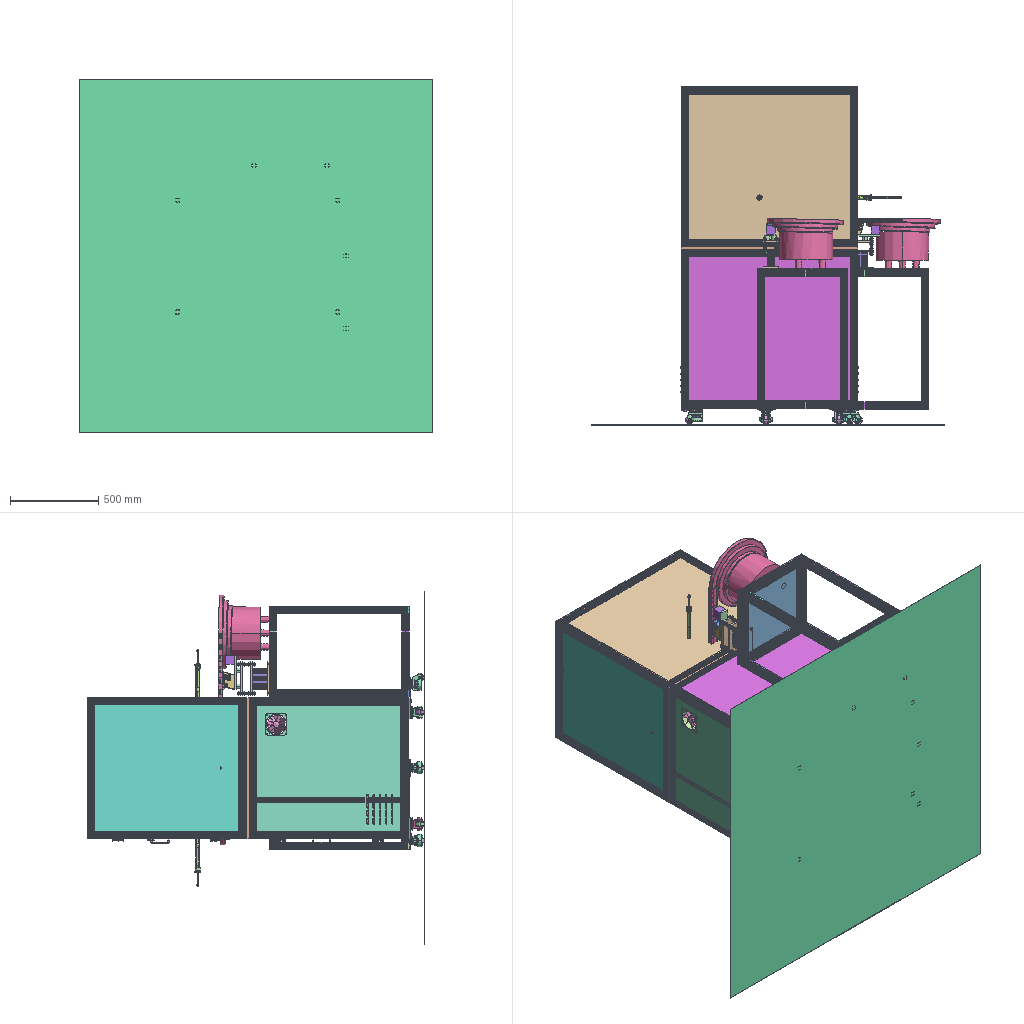Assembly | STEP file | 130 different items | 445 placed | box 2000 x 1911 x 2000 mm
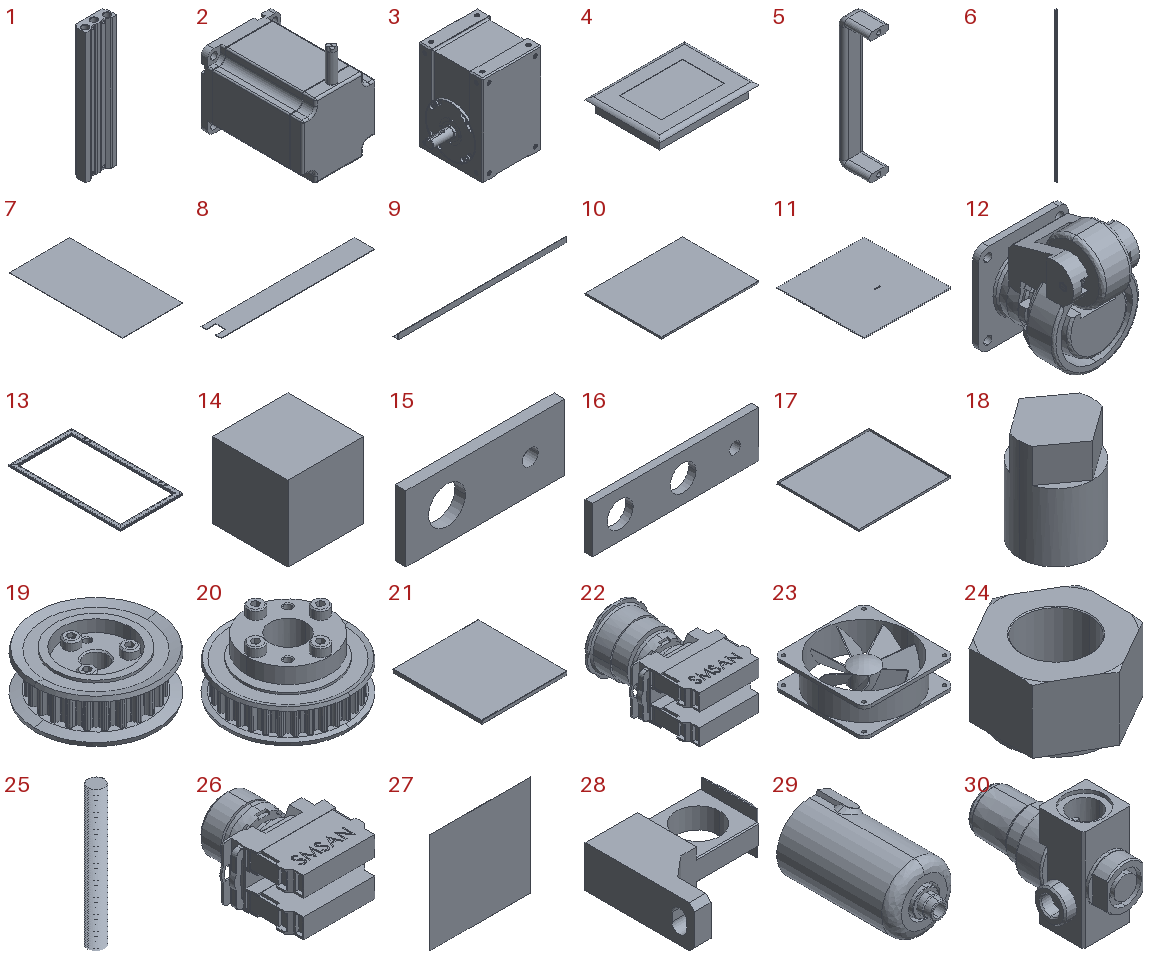Parts list (item | name | quantity | parent item | size | volume):
1 | 200M10F AirTAC base | x1 | in Solenoid valve group | 60 x 24 x 251 mm | 220028 mm3
2 | 57系列三相混合式步进电机[573S15]大国工匠 | x1 | in Material mechanism | 57.15 x 100 x 81.15 mm | 232236 mm3
3 | 60DF cam indexer | x1 | in Material mechanism | 190 x 140 x 170 mm | 2161358 mm3
4 | 7-inch Weintek touch screen TH765-N[7-inch Weintek touch screen TH765-N]_7-inch Weintek touch screen TH765-N | x1 | in Frame assembly | 213 x 159 x 46.5 mm | 1006657 mm3
5 | AKM01-96 handle | x3 | in Frame assembly | 15.6 x 25 x 102 mm | 11694 mm3
6 | AMH71封条-408 | x2 | in Frame assembly | 10.8 x 17.5 x 720 mm | 56736 mm3
7 | Acrylic cabinet door | x3 | in Frame assembly | 418.495 x 778.997 x 2 mm | 652013 mm3
8 | Acrylic cover plate | x2 | in Vibratory feeder mechanism, Vibratory feeder mechanism- | 315 x 41 x 1 mm | 12515 mm3
9 | Angle steel_Default<machined> | x2 | in Frame assembly | 960 x 30 x 30 mm | 210971 mm3
10 | Base plate | x1 | in Frame assembly | 919 x 719 x 16.2 mm | 850250 mm3
11 | Bass plate | x1 | in Material mechanism | 800 x 800 x 8 mm | 5115227 mm3
12 | CGR51-60-U Fuma caster | x2 | in Frame assembly | 73 x 81.5 x 99 mm | 226029 mm3
13 | Cabinet door_Default<machined> | x1 | in Frame assembly | 457.5 x 818 x 15 mm | 630876 mm3
14 | Collection box | x1 | in Hinge assembly equipment | 150 x 150 x 150 mm | 220232 mm3
15 | Connecting plate | x2 | in Handling mechanism | 60 x 4 x 25 mm | 5271 mm3
16 | Connecting plate 2 | x1 | in Station 4 mechanism | 90 x 4 x 25 mm | 7655 mm3
17 | Cover plate | x1 | in Frame assembly | 918 x 818 x 20 mm | 977655 mm3
18 | Diamond pin | x8 | in Material mechanism | 6.5 x 6.5 x 9 mm | 250.881 mm3
19 | ECC05-S5M100-24-F-d8 stepper motor timing pulley | x1 | in Material mechanism | 45 x 45 x 16 mm | 14077 mm3
20 | ECC05-S5M100-32-E-d16 | x1 | in Material mechanism | 55 x 55 x 29 mm | 33207 mm3
21 | Electrical plate | x1 | in Frame assembly | 337.193 x 351.476 x 13.2 mm | 161258 mm3
22 | Emergency stop button[QG115-A1-01ZS╱R] | x1 | in Frame assembly | 48.3 x 74.961 x 39.345 mm | 58947 mm3
23 | Fan[Fan]_Fan | x2 | in Frame assembly | 120 x 120 x 40.344 mm | 86776 mm3
24 | GB/T1229-1991 high-strength heavy hex nut for steel structures M12 | x32 | in Vibratory feeder mechanism, Vibratory feeder mechanism- | 19.773 x 22.78 x 12.3 mm | 2715 mm3
25 | GB/T15389-1994 screw rod M12×100 | x8 | in Vibratory feeder mechanism, Vibratory feeder mechanism- | 12 x 12 x 100 mm | 9042 mm3
26 | Green button[QG115-A2-10TD╱G] | x1 | in Frame assembly | 48.3 x 61.9 x 30.1 mm | 44921 mm3
27 | Ground | x1 | in Hinge assembly equipment | 2000 x 2 x 2000 mm | 8000000 mm3
28 | HI_BC4000 Br | x2 | in BC4000 (FRL unit) | 60 x 52.5 x 20 mm | 24751 mm3
29 | HI_BF4000-A By | x1 | in BC4000 (FRL unit) | 54.5 x 108 x 57.228 mm | 40033 mm3
30 | HI_BR4000 By-BR | x1 | in BC4000 (FRL unit) | 44 x 86.3 x 63 mm | 87528 mm3
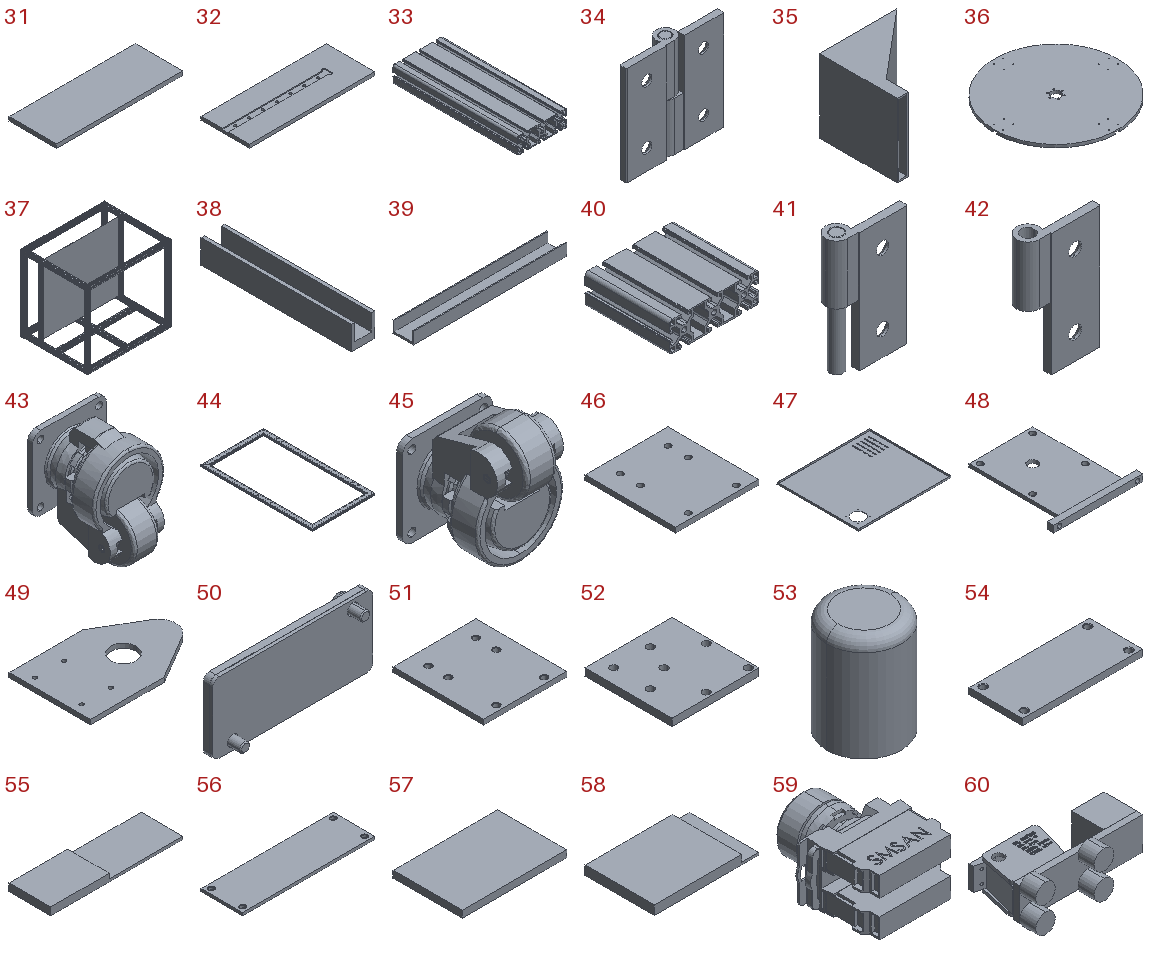31 | Handling mechanism base plate | x3 | in Handling mechanism, Station 4 mechanism | 160 x 60 x 5 mm | 48000 mm3
32 | Handling mechanism support plate | x3 | in Handling mechanism, Station 4 mechanism | 181.74 x 70 x 5 mm | 61345 mm3
33 | Handling mechanism support_Default<machined> | x3 | in Handling mechanism, Station 4 mechanism | 120 x 300 x 40 mm | 478423 mm3
34 | Hinge assembly | x2 | in Hinge assembly equipment, Material mechanism | 62 x 12.05 x 63 mm | 18899 mm3
35 | Hopper | x1 | in Station 3 mechanism | 69.588 x 70 x 66 mm | 22407 mm3
36 | Indexing plate | x1 | in Material mechanism | 450 x 450 x 12 mm | 1702254 mm3
37 | Lower frame_aluminium extrusion<machined> | x1 | in Frame assembly | 1000 x 800 x 900 mm | 9363602 mm3
38 | Magazine box | x1 | in Station 3 mechanism | 10 x 63 x 10 mm | 3213 mm3
39 | Material chute | x2 | in Vibratory feeder mechanism, Vibratory feeder mechanism- | 315 x 41 x 24 mm | 76860 mm3
40 | Material transfer mechanism support_Default<machined> | x2 | in Material transfer mechanism, Material transfer mechanism- | 120 x 112.995 x 40 mm | 180199 mm3
41 | Mirror _AKQ01-B-Z-R-6263-001 | x2 | in Mirrored AKQ01 hinge | 36.75 x 12.05 x 63 mm | 10659 mm3
42 | Mirror _AKQ01-B-Z-R-6263-002 | x2 | in Mirrored AKQ01 hinge | 36.75 x 12.05 x 63 mm | 8240 mm3
43 | Mirrored CGR51-60-U Fuma caster | x1 | in Frame assembly | 73 x 81.5 x 99 mm | 226024 mm3
44 | Mirrored cabinet door_Default<machined> | x2 | in Frame assembly | 457.5 x 818 x 15 mm | 630876 mm3
45 | Mirrored mirrored CGR51-60-U Fuma caster | x1 | in Frame assembly | 73 x 81.5 x 99 mm | 226029 mm3
46 | Mirrored pad plate | x2 | in Vibratory bowl feeder support mechanism | 100.5 x 110 x 6 mm | 64996 mm3
47 | Mirrored side cover plate1_mirror | x1 | in Frame assembly | 818 x 718 x 22.2 mm | 748491 mm3
48 | Motor mounting plate | x1 | in Material mechanism | 80 x 87.326 x 6 mm | 16246 mm3
49 | Mounting plate | x3 | in Handling mechanism, Station 4 mechanism | 108.5 x 70 x 4 mm | 23874 mm3
50 | P-200M-R2 AirTAC base blind plate assembly | x1 | in Solenoid valve group | 50.7 x 9 x 22.4 mm | 3480 mm3
51 | Pad plate | x2 | in Vibratory bowl feeder support mechanism | 100.5 x 110 x 6 mm | 64996 mm3
52 | Pad plate- | x4 | in Frame assembly | 120 x 120 x 10 mm | 138500 mm3
53 | Pin | x8 | in Material mechanism | 6.5 x 6.5 x 9 mm | 259.622 mm3
54 | Plate | x6 | in Vibratory feeder mechanism, Vibratory feeder mechanism- | 190 x 85 x 10 mm | 158173 mm3
55 | Plate 1 | x2 | in Material transfer mechanism, Material transfer mechanism- | 190 x 60 x 11 mm | 80880 mm3
56 | Plate 2 | x2 | in Material transfer mechanism, Material transfer mechanism- | 190 x 60 x 4 mm | 45001 mm3
57 | Plate 3 | x1 | in Station 3 mechanism | 91 x 60 x 6 mm | 32760 mm3
58 | Plate 4 | x1 | in Station 3 mechanism | 91 x 60 x 8 mm | 38280 mm3
59 | Red button[QG115-A2-10TD╱R] | x1 | in Frame assembly | 48.3 x 61.9 x 30.1 mm | 44921 mm3
60 | SKC-PZ-100 counterweight vibratory feeder | x2 | in Vibratory feeder mechanism, Vibratory feeder mechanism- | - | 385547 mm3
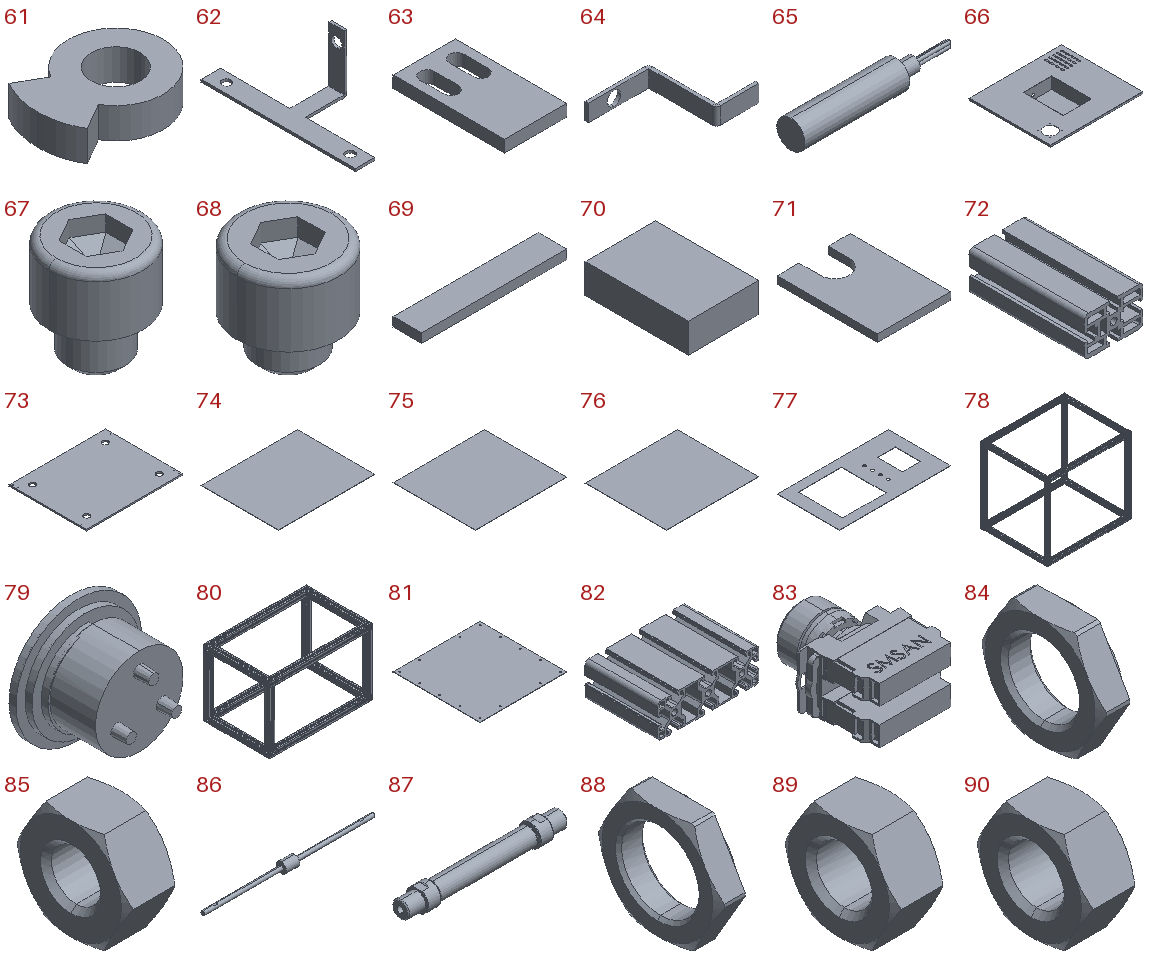61 | Sensing plate | x1 | in Material mechanism | 41 x 31 x 10 mm | 7684 mm3
62 | Sensor bracket | x1 | in Material mechanism | 47.2 x 120 x 45 mm | 5138 mm3
63 | Sensor spacer block | x2 | in Material transfer mechanism, Material transfer mechanism- | 21 x 37.576 x 4 mm | 2679 mm3
64 | Sensor support | x2 | in Material transfer mechanism, Material transfer mechanism- | 60.39 x 42 x 10 mm | 1887 mm3
65 | Sensors | x3 | in Material mechanism, Material transfer mechanism, Material transfer mechanism- | 45 x 8 x 8 mm | 1594 mm3
66 | Side cover plate | x1 | in Frame assembly | 818 x 718 x 108.6 mm | 888983 mm3
67 | Socket head cap screw M10x8 | x12 | in Frame assembly | 16 x 16 x 18 mm | 2409 mm3
68 | Socket head cap screw M8x5 | x16 | in Frame assembly | 13 x 13 x 13 mm | 1204 mm3
69 | Spacer block | x2 | in Station 1 feeding mechanism, Station 2 mechanism | 126 x 24.75 x 7.95 mm | 24792 mm3
70 | Spacer block 4 | x3 | in Handling mechanism, Station 4 mechanism | 48 x 70 x 20 mm | 67200 mm3
71 | Station 3 cylinder connecting plate | x1 | in Station 3 mechanism | 40 x 55 x 4 mm | 7662 mm3
72 | Station 3 support_Default<machined> | x1 | in Station 3 mechanism | 60 x 118.295 x 40 mm | 132045 mm3
73 | Top plate | x1 | in Frame assembly | 1000 x 800 x 14 mm | 11039590 mm3
74 | Upper cover plate | x1 | in Frame assembly | 1000 x 800 x 3 mm | 2399999 mm3
75 | Upper frame acrylic cover plate | x1 | in Frame assembly | 948.003 x 848 x 2 mm | 1607813 mm3
76 | Upper frame acrylic side plate | x2 | in Frame assembly | 848.001 x 747.917 x 2 mm | 1268468 mm3
77 | Upper frame door panel | x1 | in Frame assembly | 848 x 474.5 x 2 mm | 525505 mm3
78 | Upper frame_Default<machined> | x1 | in Frame assembly | 1000 x 800 x 900 mm | 6810900 mm3
79 | Vibratory bowl feeder | x2 | in Station 1 feeding mechanism, Station 2 mechanism | 416.592 x 286.08 x 431.538 mm | 12004626 mm3
80 | Vibratory bowl feeder support frame_Default<machined> | x2 | in Vibratory bowl feeder support mechanism | 790 x 510 x 510 mm | 4425071 mm3
81 | Vibratory bowl feeder support plate | x2 | in Vibratory bowl feeder support mechanism | 509.5 x 510 x 2 mm | 518611 mm3
82 | Vibratory feeder support_Default<machined> | x2 | in Vibratory feeder mechanism, Vibratory feeder mechanism- | 120 x 86.083 x 40 mm | 137280 mm3
83 | Yellow button[QG115-A2-10TD╱Y] | x1 | in Frame assembly | 48.3 x 61.9 x 30.1 mm | 44921 mm3
84 | _16 MA Nut | x2 | - | 6 x 25 x 22 mm | 1467 mm3
85 | _16 MA Nut1 | x1 | - | 5 x 11.547 x 10 mm | 331.011 mm3
86 | _16MAD600Rod | x1 | - | 256 x 15.5 x 15.5 mm | 10417 mm3
87 | _16MAD60Body | x1 | - | 152 x 21 x 21 mm | 19082 mm3
88 | _20 MA Nut | x6 | - | 7 x 33 x 29 mm | 2695 mm3
89 | _20 MA Nut1 | x3 | - | 6 x 13.856 x 12 mm | 526.038 mm3
90 | _20 MAJ Nut | x3 | - | 6 x 13.856 x 12 mm | 526.038 mm3
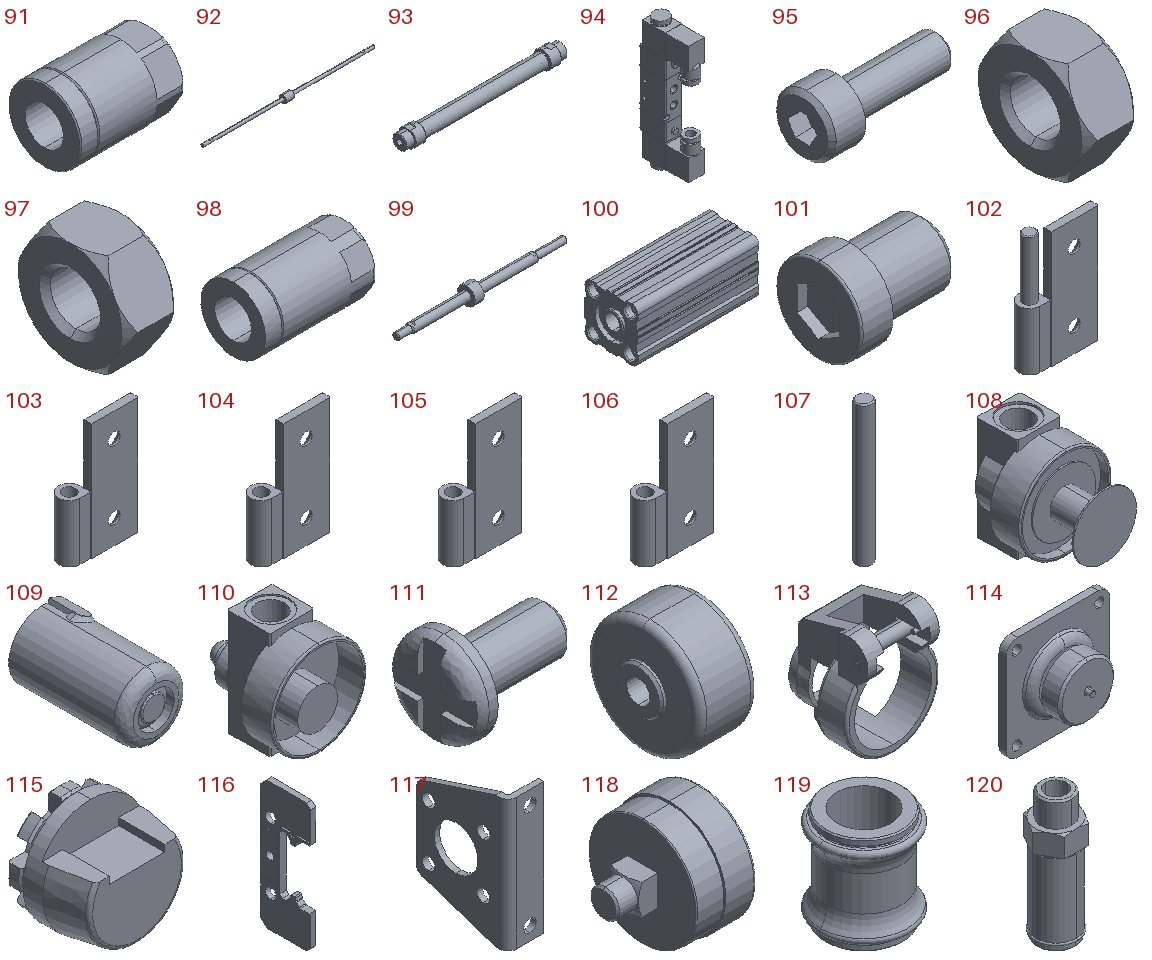91 | _20MACJ15010A-Nut | x3 | - | 29 x 20 x 20 mm | 7030 mm3
92 | _20MACJ15010Rod | x3 | - | 463 x 19.5 x 19.5 mm | 28625 mm3
93 | _20MACJ150Body | x3 | - | 250 x 27 x 27 mm | 37841 mm3
94 | _4V220-06(By).stp | x9 | in 4V22006B AirTAC solenoid valve.stp | 22 x 66.8 x 171.8 mm | 158549 mm3
95 | _ACQJ 16 - LB - Screw | x40 | - | 16 x 7 x 7 mm | 285.452 mm3
96 | _ACQJ 16_Ad_Nut | x5 | in Assembly 1 | 5 x 11.547 x 10 mm | 329.448 mm3
97 | _ACQJ 16_Nut | x5 | in Assembly 1 | 5 x 11.547 x 10 mm | 329.448 mm3
98 | _ACQJ-16x10_stoper | x5 | in Assembly 1 | 26 x 15 x 15 mm | 3348 mm3
99 | _ACQJ-16x40-B10_r(40-10) | x5 | in Assembly 1 | 152.5 x 16 x 16 mm | 7956 mm3
100 | _ACQJ-16x40-B_b (40) | x5 | - | 66 x 29 x 29 mm | 38011 mm3
101 | _AFC1500 Sc | x2 | in BC4000 (FRL unit) | 10 x 8 x 8 mm | 331.348 mm3
102 | _AKQ01-B-Z-R-6263-001 | x4 | in AKQ01 hinge | 36.75 x 12.05 x 63 mm | 10659 mm3
103 | _AKQ01-B-Z-R-6263-002 | x4 | in AKQ01 hinge | 36.75 x 12.05 x 63 mm | 8240 mm3
104 | _AKQ01怡合达合页1 | x7 | in Material mechanism, Station 1 feeding mechanism, Station 2 mechanism | 36.75 x 12.05 x 63 mm | 8240 mm3
105 | _AKQ01怡合达合页1- | x10 | in Vibratory feeder mechanism, Vibratory feeder mechanism- | 36.75 x 12.05 x 63 mm | 8240 mm3
106 | _AKQ01怡合达合页2- | x2 | in Material transfer mechanism, Material transfer mechanism- | 36.75 x 12.05 x 63 mm | 8240 mm3
107 | _AKQ01怡合达销1 | x21 | in Station 3 mechanism | 7 x 7 x 63 mm | 2419 mm3
108 | _BF4000 Sw | x1 | in BC4000 (FRL unit) | 64 x 74.25 x 72 mm | 119658 mm3
109 | _BL-4000 By | x1 | in BC4000 (FRL unit) | 54.5 x 95.3 x 57.228 mm | 39272 mm3
110 | _BL-4000 Sw | x1 | in BC4000 (FRL unit) | 64 x 69.32 x 72 mm | 89554 mm3
111 | _Bolt-MG9 | x12 | in Assembly 4 | 4 x 3 x 3 mm | 10.872 mm3
112 | _CGR51-60-U-001.stp | x4 | in Yiheda Fuma caster.stp | 29 x 49 x 49 mm | 45483 mm3
113 | _CGR51-60-U-002.stp | x4 | in Yiheda Fuma caster.stp | 70 x 63 x 89.5 mm | 67213 mm3
114 | _CGR51-60-U-003.stp | x4 | in Yiheda Fuma caster.stp | 73 x 29.8 x 73 mm | 47628 mm3
115 | _CGR51-60-U-004.stp | x4 | in Yiheda Fuma caster.stp | 55 x 39.5 x 55 mm | 65697 mm3
116 | _EndSeal-MGN9 | x6 | in Assembly 4 | 1 x 7.7 x 19.6 mm | 85.449 mm3
117 | _F-ACQ16LB | x10 | - | 13 x 33.5 x 48 mm | 3042 mm3
118 | _GS-50 GaUGE | x1 | in BC4000 (FRL unit) | 44.5 x 52 x 52 mm | 55461 mm3
119 | _HSV10 -slide.stp | x1 | in HSV10 AirTAC hand slide valve.stp | 35.5 x 35.5 x 39 mm | 15226 mm3
120 | _HSV10 Body.stp | x1 | in HSV10 AirTAC hand slide valve.stp | 25.403 x 22.74 x 68.5 mm | 19346 mm3
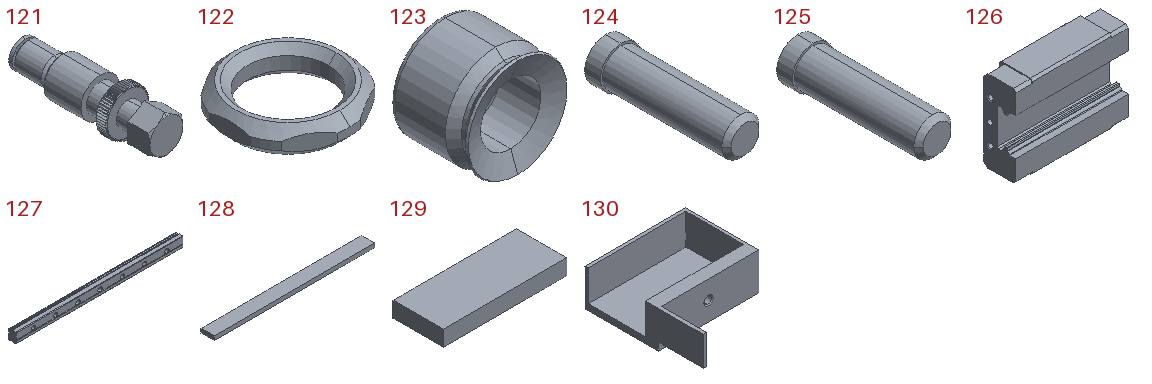121 | _J-WES26-d10-001 | x4 | in Yiheda vacuum suction cup | 16 x 52.1 x 16.9 mm | 5380 mm3
122 | _J-WES26-d10-002 | x8 | in Yiheda vacuum suction cup | 17 x 18 x 4 mm | 405.758 mm3
123 | _J-WES26-d10-003 | x4 | in Yiheda vacuum suction cup | 10 x 7.688 x 10 mm | 388.501 mm3
124 | _MG-P-Screw-9-N | x3 | in Assembly 4 | 1.333 x 4.5 x 1.333 mm | 5.111 mm3
125 | _MG-Plug-Screw-9-N | x3 | in Assembly 4 | 1.333 x 4.5 x 1.333 mm | 5.052 mm3
126 | _MGN9CZ0HM | x3 | in Assembly 4 | 26.9 x 8 x 20 mm | 3027 mm3
127 | _Rail-MGN9R01501HM-7.5 | x3 | in MGN9 HIWIN rail C1R0150Z0HM-No-Set-E1_7.5 | 150 x 6.5 x 9 mm | 7402 mm3
128 | 垫块1- | x2 | in Vibratory feeder mechanism, Vibratory feeder mechanism- | 315 x 25.5 x 7.95 mm | 63858 mm3
129 | 垫块5- | x2 | in Material transfer mechanism, Material transfer mechanism- | 63 x 25.5 x 7.95 mm | 12772 mm3
130 | 料槽1 | x2 | in Material transfer mechanism, Material transfer mechanism- | 65 x 76 x 24 mm | 27672 mm3